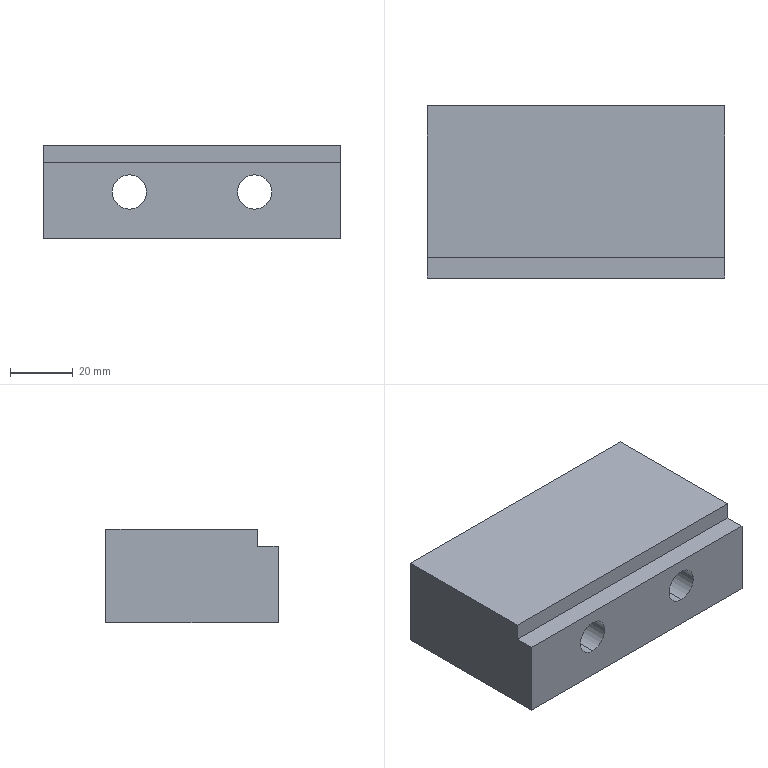Part | SolidWorks | features ICE 3, Extrusion 1 | 1 solid | 18 faces | box 95 x 55 x 30 mm | volume 136523 mm3 | plane 10 | cylinder 8 | commonest cylinder face diameters 11 x4 18 x4
STEP:
#1=CARTESIAN_POINT('',(20.,35.,-9.));
#2=VERTEX_POINT('',#1);
#3=CARTESIAN_POINT('',(20.,35.,9.));
#4=VERTEX_POINT('',#3);
#5=CARTESIAN_POINT('',(20.,35.,0.));
#6=DIRECTION('',(0.,1.,0.));
#7=DIRECTION('',(0.,0.,1.));
#8=AXIS2_PLACEMENT_3D('',#5,#6,#7);
#9=CIRCLE('',#8,9.);
#10=EDGE_CURVE('',#2,#4,#9,.T.);
#11=ORIENTED_EDGE('',*,*,#10,.F.);
#12=CARTESIAN_POINT('',(20.,55.,-9.));
#13=VERTEX_POINT('',#12);
#14=CARTESIAN_POINT('',(20.,35.,-9.));
#15=DIRECTION('',(0.,1.,0.));
#16=VECTOR('',#15,1000.);
#17=LINE('',#14,#16);
#18=EDGE_CURVE('',#2,#13,#17,.T.);
#19=ORIENTED_EDGE('',*,*,#18,.T.);
#20=CARTESIAN_POINT('',(20.,55.,9.));
#21=VERTEX_POINT('',#20);
#22=CARTESIAN_POINT('',(20.,55.,0.));
#23=DIRECTION('',(0.,1.,0.));
#24=DIRECTION('',(0.,0.,1.));
#25=AXIS2_PLACEMENT_3D('',#22,#23,#24);
#26=CIRCLE('',#25,9.);
#27=EDGE_CURVE('',#13,#21,#26,.T.);
#28=ORIENTED_EDGE('',*,*,#27,.T.);
#29=CARTESIAN_POINT('',(20.,35.,9.));
#30=DIRECTION('',(0.,1.,0.));
#31=VECTOR('',#30,1000.);
#32=LINE('',#29,#31);
#33=EDGE_CURVE('',#4,#21,#32,.T.);
#34=ORIENTED_EDGE('',*,*,#33,.F.);
#35=EDGE_LOOP('',(#11,#19,#28,#34));
#36=FACE_OUTER_BOUND('',#35,.T.);
#37=CARTESIAN_POINT('',(20.,35.,0.));
#38=DIRECTION('',(0.,1.,0.));
#39=DIRECTION('',(0.,0.,1.));
#40=AXIS2_PLACEMENT_3D('',#37,#38,#39);
#41=CYLINDRICAL_SURFACE('',#40,9.);
#42=ADVANCED_FACE('',(#36),#41,.F.);
#43=CARTESIAN_POINT('',(-20.,35.,-9.));
#44=VERTEX_POINT('',#43);
#45=CARTESIAN_POINT('',(-20.,35.,9.));
#46=VERTEX_POINT('',#45);
#47=CARTESIAN_POINT('',(-20.,35.,0.));
#48=DIRECTION('',(0.,1.,0.));
#49=DIRECTION('',(0.,0.,1.));
#50=AXIS2_PLACEMENT_3D('',#47,#48,#49);
#51=CIRCLE('',#50,9.);
#52=EDGE_CURVE('',#44,#46,#51,.T.);
#53=ORIENTED_EDGE('',*,*,#52,.F.);
#54=CARTESIAN_POINT('',(-20.,55.,-9.));
#55=VERTEX_POINT('',#54);
#56=CARTESIAN_POINT('',(-20.,35.,-9.));
#57=DIRECTION('',(0.,1.,0.));
#58=VECTOR('',#57,1000.);
#59=LINE('',#56,#58);
#60=EDGE_CURVE('',#44,#55,#59,.T.);
#61=ORIENTED_EDGE('',*,*,#60,.T.);
#62=CARTESIAN_POINT('',(-20.,55.,9.));
#63=VERTEX_POINT('',#62);
#64=CARTESIAN_POINT('',(-20.,55.,0.));
#65=DIRECTION('',(0.,1.,0.));
#66=DIRECTION('',(0.,0.,1.));
#67=AXIS2_PLACEMENT_3D('',#64,#65,#66);
#68=CIRCLE('',#67,9.);
#69=EDGE_CURVE('',#55,#63,#68,.T.);
#70=ORIENTED_EDGE('',*,*,#69,.T.);
#71=CARTESIAN_POINT('',(-20.,35.,9.));
#72=DIRECTION('',(0.,1.,0.));
#73=VECTOR('',#72,1000.);
#74=LINE('',#71,#73);
#75=EDGE_CURVE('',#46,#63,#74,.T.);
#76=ORIENTED_EDGE('',*,*,#75,.F.);
#77=EDGE_LOOP('',(#53,#61,#70,#76));
#78=FACE_OUTER_BOUND('',#77,.T.);
#79=CARTESIAN_POINT('',(-20.,35.,0.));
#80=DIRECTION('',(0.,1.,0.));
#81=DIRECTION('',(0.,0.,1.));
#82=AXIS2_PLACEMENT_3D('',#79,#80,#81);
#83=CYLINDRICAL_SURFACE('',#82,9.);
#84=ADVANCED_FACE('',(#78),#83,.F.);
#85=CARTESIAN_POINT('',(-20.,0.,-5.5));
#86=VERTEX_POINT('',#85);
#87=CARTESIAN_POINT('',(-20.,0.,5.5));
#88=VERTEX_POINT('',#87);
#89=CARTESIAN_POINT('',(-20.,0.,0.));
#90=DIRECTION('',(0.,1.,0.));
#91=DIRECTION('',(0.,0.,1.));
#92=AXIS2_PLACEMENT_3D('',#89,#90,#91);
#93=CIRCLE('',#92,5.5);
#94=EDGE_CURVE('',#86,#88,#93,.T.);
#95=ORIENTED_EDGE('',*,*,#94,.F.);
#96=CARTESIAN_POINT('',(-20.,35.,-5.5));
#97=VERTEX_POINT('',#96);
#98=CARTESIAN_POINT('',(-20.,0.,-5.5));
#99=DIRECTION('',(0.,1.,0.));
#100=VECTOR('',#99,1000.);
#101=LINE('',#98,#100);
#102=EDGE_CURVE('',#86,#97,#101,.T.);
#103=ORIENTED_EDGE('',*,*,#102,.T.);
#104=CARTESIAN_POINT('',(-20.,35.,5.5));
#105=VERTEX_POINT('',#104);
#106=CARTESIAN_POINT('',(-20.,35.,0.));
#107=DIRECTION('',(0.,-1.,0.));
#108=DIRECTION('',(0.,0.,1.));
#109=AXIS2_PLACEMENT_3D('',#106,#107,#108);
#110=CIRCLE('',#109,5.5);
#111=EDGE_CURVE('',#105,#97,#110,.T.);
#112=ORIENTED_EDGE('',*,*,#111,.F.);
#113=CARTESIAN_POINT('',(-20.,0.,5.5));
#114=DIRECTION('',(0.,1.,0.));
#115=VECTOR('',#114,1000.);
#116=LINE('',#113,#115);
#117=EDGE_CURVE('',#88,#105,#116,.T.);
#118=ORIENTED_EDGE('',*,*,#117,.F.);
#119=EDGE_LOOP('',(#95,#103,#112,#118));
#120=FACE_OUTER_BOUND('',#119,.T.);
#121=CARTESIAN_POINT('',(-20.,0.,0.));
#122=DIRECTION('',(0.,1.,0.));
#123=DIRECTION('',(0.,0.,1.));
#124=AXIS2_PLACEMENT_3D('',#121,#122,#123);
#125=CYLINDRICAL_SURFACE('',#124,5.5);
#126=ADVANCED_FACE('',(#120),#125,.F.);
#127=CARTESIAN_POINT('',(20.,0.,-5.5));
#128=VERTEX_POINT('',#127);
#129=CARTESIAN_POINT('',(20.,0.,5.5));
#130=VERTEX_POINT('',#129);
#131=CARTESIAN_POINT('',(20.,0.,0.));
#132=DIRECTION('',(0.,1.,0.));
#133=DIRECTION('',(0.,0.,1.));
#134=AXIS2_PLACEMENT_3D('',#131,#132,#133);
#135=CIRCLE('',#134,5.5);
#136=EDGE_CURVE('',#128,#130,#135,.T.);
#137=ORIENTED_EDGE('',*,*,#136,.F.);
#138=CARTESIAN_POINT('',(20.,35.,-5.5));
#139=VERTEX_POINT('',#138);
#140=CARTESIAN_POINT('',(20.,0.,-5.5));
#141=DIRECTION('',(0.,1.,0.));
#142=VECTOR('',#141,1000.);
#143=LINE('',#140,#142);
#144=EDGE_CURVE('',#128,#139,#143,.T.);
#145=ORIENTED_EDGE('',*,*,#144,.T.);
#146=CARTESIAN_POINT('',(20.,35.,5.5));
#147=VERTEX_POINT('',#146);
#148=CARTESIAN_POINT('',(20.,35.,0.));
#149=DIRECTION('',(0.,-1.,0.));
#150=DIRECTION('',(0.,0.,1.));
#151=AXIS2_PLACEMENT_3D('',#148,#149,#150);
#152=CIRCLE('',#151,5.5);
#153=EDGE_CURVE('',#147,#139,#152,.T.);
#154=ORIENTED_EDGE('',*,*,#153,.F.);
#155=CARTESIAN_POINT('',(20.,0.,5.5));
#156=DIRECTION('',(0.,1.,0.));
#157=VECTOR('',#156,1000.);
#158=LINE('',#155,#157);
#159=EDGE_CURVE('',#130,#147,#158,.T.);
#160=ORIENTED_EDGE('',*,*,#159,.F.);
#161=EDGE_LOOP('',(#137,#145,#154,#160));
#162=FACE_OUTER_BOUND('',#161,.T.);
#163=CARTESIAN_POINT('',(20.,0.,0.));
#164=DIRECTION('',(0.,1.,0.));
#165=DIRECTION('',(0.,0.,1.));
#166=AXIS2_PLACEMENT_3D('',#163,#164,#165);
#167=CYLINDRICAL_SURFACE('',#166,5.5);
#168=ADVANCED_FACE('',(#162),#167,.F.);
#169=ORIENTED_EDGE('',*,*,#144,.F.);
#170=CARTESIAN_POINT('',(20.,0.,0.));
#171=DIRECTION('',(0.,1.,0.));
#172=DIRECTION('',(0.,0.,1.));
#173=AXIS2_PLACEMENT_3D('',#170,#171,#172);
#174=CIRCLE('',#173,5.5);
#175=EDGE_CURVE('',#130,#128,#174,.T.);
#176=ORIENTED_EDGE('',*,*,#175,.F.);
#177=ORIENTED_EDGE('',*,*,#159,.T.);
#178=CARTESIAN_POINT('',(20.,35.,0.));
#179=DIRECTION('',(0.,-1.,0.));
#180=DIRECTION('',(0.,0.,1.));
#181=AXIS2_PLACEMENT_3D('',#178,#179,#180);
#182=CIRCLE('',#181,5.5);
#183=EDGE_CURVE('',#139,#147,#182,.T.);
#184=ORIENTED_EDGE('',*,*,#183,.F.);
#185=EDGE_LOOP('',(#169,#176,#177,#184));
#186=FACE_OUTER_BOUND('',#185,.T.);
#187=CARTESIAN_POINT('',(20.,0.,0.));
#188=DIRECTION('',(0.,1.,0.));
#189=DIRECTION('',(0.,0.,1.));
#190=AXIS2_PLACEMENT_3D('',#187,#188,#189);
#191=CYLINDRICAL_SURFACE('',#190,5.5);
#192=ADVANCED_FACE('',(#186),#191,.F.);
#193=ORIENTED_EDGE('',*,*,#102,.F.);
#194=CARTESIAN_POINT('',(-20.,0.,0.));
#195=DIRECTION('',(0.,1.,0.));
#196=DIRECTION('',(0.,0.,1.));
#197=AXIS2_PLACEMENT_3D('',#194,#195,#196);
#198=CIRCLE('',#197,5.5);
#199=EDGE_CURVE('',#88,#86,#198,.T.);
#200=ORIENTED_EDGE('',*,*,#199,.F.);
#201=ORIENTED_EDGE('',*,*,#117,.T.);
#202=CARTESIAN_POINT('',(-20.,35.,0.));
#203=DIRECTION('',(0.,-1.,0.));
#204=DIRECTION('',(0.,0.,1.));
#205=AXIS2_PLACEMENT_3D('',#202,#203,#204);
#206=CIRCLE('',#205,5.5);
#207=EDGE_CURVE('',#97,#105,#206,.T.);
#208=ORIENTED_EDGE('',*,*,#207,.F.);
#209=EDGE_LOOP('',(#193,#200,#201,#208));
#210=FACE_OUTER_BOUND('',#209,.T.);
#211=CARTESIAN_POINT('',(-20.,0.,0.));
#212=DIRECTION('',(0.,1.,0.));
#213=DIRECTION('',(0.,0.,1.));
#214=AXIS2_PLACEMENT_3D('',#211,#212,#213);
#215=CYLINDRICAL_SURFACE('',#214,5.5);
#216=ADVANCED_FACE('',(#210),#215,.F.);
#217=CARTESIAN_POINT('',(47.5,6.5,15.));
#218=VERTEX_POINT('',#217);
#219=CARTESIAN_POINT('',(47.5,6.5,9.5));
#220=VERTEX_POINT('',#219);
#221=CARTESIAN_POINT('',(47.5,6.5,15.));
#222=DIRECTION('',(0.,0.,-1.));
#223=VECTOR('',#222,1000.);
#224=LINE('',#221,#223);
#225=EDGE_CURVE('',#218,#220,#224,.T.);
#226=ORIENTED_EDGE('',*,*,#225,.T.);
#227=CARTESIAN_POINT('',(47.5,0.,9.5));
#228=VERTEX_POINT('',#227);
#229=CARTESIAN_POINT('',(47.5,55.,9.5));
#230=DIRECTION('',(0.,-1.,0.));
#231=VECTOR('',#230,1000.);
#232=LINE('',#229,#231);
#233=EDGE_CURVE('',#220,#228,#232,.T.);
#234=ORIENTED_EDGE('',*,*,#233,.T.);
#235=CARTESIAN_POINT('',(47.5,0.,-15.));
#236=VERTEX_POINT('',#235);
#237=CARTESIAN_POINT('',(47.5,0.,15.));
#238=DIRECTION('',(0.,0.,-1.));
#239=VECTOR('',#238,1000.);
#240=LINE('',#237,#239);
#241=EDGE_CURVE('',#228,#236,#240,.T.);
#242=ORIENTED_EDGE('',*,*,#241,.T.);
#243=CARTESIAN_POINT('',(47.5,55.,-15.));
#244=VERTEX_POINT('',#243);
#245=CARTESIAN_POINT('',(47.5,55.,-15.));
#246=DIRECTION('',(0.,-1.,0.));
#247=VECTOR('',#246,1000.);
#248=LINE('',#245,#247);
#249=EDGE_CURVE('',#244,#236,#248,.T.);
#250=ORIENTED_EDGE('',*,*,#249,.F.);
#251=CARTESIAN_POINT('',(47.5,55.,15.));
#252=VERTEX_POINT('',#251);
#253=CARTESIAN_POINT('',(47.5,55.,15.));
#254=DIRECTION('',(0.,0.,-1.));
#255=VECTOR('',#254,1000.);
#256=LINE('',#253,#255);
#257=EDGE_CURVE('',#252,#244,#256,.T.);
#258=ORIENTED_EDGE('',*,*,#257,.F.);
#259=CARTESIAN_POINT('',(47.5,55.,15.));
#260=DIRECTION('',(0.,-1.,0.));
#261=VECTOR('',#260,1000.);
#262=LINE('',#259,#261);
#263=EDGE_CURVE('',#252,#218,#262,.T.);
#264=ORIENTED_EDGE('',*,*,#263,.T.);
#265=EDGE_LOOP('',(#226,#234,#242,#250,#258,#264));
#266=FACE_OUTER_BOUND('',#265,.T.);
#267=CARTESIAN_POINT('',(47.5,55.,15.));
#268=DIRECTION('',(-1.,0.,0.));
#269=DIRECTION('',(0.,0.,1.));
#270=AXIS2_PLACEMENT_3D('',#267,#268,#269);
#271=PLANE('',#270);
#272=ADVANCED_FACE('',(#266),#271,.F.);
#273=CARTESIAN_POINT('',(-47.5,0.,-15.));
#274=VERTEX_POINT('',#273);
#275=CARTESIAN_POINT('',(-47.5,0.,-15.));
#276=DIRECTION('',(-1.,0.,0.));
#277=VECTOR('',#276,1000.);
#278=LINE('',#275,#277);
#279=EDGE_CURVE('',#236,#274,#278,.T.);
#280=ORIENTED_EDGE('',*,*,#279,.T.);
#281=CARTESIAN_POINT('',(-47.5,55.,-15.));
#282=VERTEX_POINT('',#281);
#283=CARTESIAN_POINT('',(-47.5,55.,-15.));
#284=DIRECTION('',(0.,-1.,0.));
#285=VECTOR('',#284,1000.);
#286=LINE('',#283,#285);
#287=EDGE_CURVE('',#282,#274,#286,.T.);
#288=ORIENTED_EDGE('',*,*,#287,.F.);
#289=CARTESIAN_POINT('',(-47.5,55.,-15.));
#290=DIRECTION('',(-1.,0.,0.));
#291=VECTOR('',#290,1000.);
#292=LINE('',#289,#291);
#293=EDGE_CURVE('',#244,#282,#292,.T.);
#294=ORIENTED_EDGE('',*,*,#293,.F.);
#295=ORIENTED_EDGE('',*,*,#249,.T.);
#296=EDGE_LOOP('',(#280,#288,#294,#295));
#297=FACE_OUTER_BOUND('',#296,.T.);
#298=CARTESIAN_POINT('',(-47.5,55.,-15.));
#299=DIRECTION('',(0.,0.,1.));
#300=DIRECTION('',(1.,0.,0.));
#301=AXIS2_PLACEMENT_3D('',#298,#299,#300);
#302=PLANE('',#301);
#303=ADVANCED_FACE('',(#297),#302,.F.);
#304=CARTESIAN_POINT('',(-47.5,0.,9.5));
#305=VERTEX_POINT('',#304);
#306=CARTESIAN_POINT('',(-47.5,0.,15.));
#307=DIRECTION('',(0.,0.,1.));
#308=VECTOR('',#307,1000.);
#309=LINE('',#306,#308);
#310=EDGE_CURVE('',#274,#305,#309,.T.);
#311=ORIENTED_EDGE('',*,*,#310,.T.);
#312=CARTESIAN_POINT('',(-47.5,6.5,9.5));
#313=VERTEX_POINT('',#312);
#314=CARTESIAN_POINT('',(-47.5,0.,9.5));
#315=DIRECTION('',(0.,-1.,0.));
#316=VECTOR('',#315,1000.);
#317=LINE('',#314,#316);
#318=EDGE_CURVE('',#313,#305,#317,.T.);
#319=ORIENTED_EDGE('',*,*,#318,.F.);
#320=CARTESIAN_POINT('',(-47.5,6.5,15.));
#321=VERTEX_POINT('',#320);
#322=CARTESIAN_POINT('',(-47.5,6.5,15.));
#323=DIRECTION('',(0.,0.,-1.));
#324=VECTOR('',#323,1000.);
#325=LINE('',#322,#324);
#326=EDGE_CURVE('',#321,#313,#325,.T.);
#327=ORIENTED_EDGE('',*,*,#326,.F.);
#328=CARTESIAN_POINT('',(-47.5,55.,15.));
#329=VERTEX_POINT('',#328);
#330=CARTESIAN_POINT('',(-47.5,55.,15.));
#331=DIRECTION('',(0.,-1.,0.));
#332=VECTOR('',#331,1000.);
#333=LINE('',#330,#332);
#334=EDGE_CURVE('',#329,#321,#333,.T.);
#335=ORIENTED_EDGE('',*,*,#334,.F.);
#336=CARTESIAN_POINT('',(-47.5,55.,15.));
#337=DIRECTION('',(0.,0.,1.));
#338=VECTOR('',#337,1000.);
#339=LINE('',#336,#338);
#340=EDGE_CURVE('',#282,#329,#339,.T.);
#341=ORIENTED_EDGE('',*,*,#340,.F.);
#342=ORIENTED_EDGE('',*,*,#287,.T.);
#343=EDGE_LOOP('',(#311,#319,#327,#335,#341,#342));
#344=FACE_OUTER_BOUND('',#343,.T.);
#345=CARTESIAN_POINT('',(-47.5,55.,15.));
#346=DIRECTION('',(1.,0.,0.));
#347=DIRECTION('',(0.,0.,-1.));
#348=AXIS2_PLACEMENT_3D('',#345,#346,#347);
#349=PLANE('',#348);
#350=ADVANCED_FACE('',(#344),#349,.F.);
#351=ORIENTED_EDGE('',*,*,#334,.T.);
#352=CARTESIAN_POINT('',(124.5,6.5,15.));
#353=DIRECTION('',(-1.,0.,0.));
#354=VECTOR('',#353,1000.);
#355=LINE('',#352,#354);
#356=EDGE_CURVE('',#218,#321,#355,.T.);
#357=ORIENTED_EDGE('',*,*,#356,.F.);
#358=ORIENTED_EDGE('',*,*,#263,.F.);
#359=CARTESIAN_POINT('',(-47.5,55.,15.));
#360=DIRECTION('',(1.,0.,0.));
#361=VECTOR('',#360,1000.);
#362=LINE('',#359,#361);
#363=EDGE_CURVE('',#329,#252,#362,.T.);
#364=ORIENTED_EDGE('',*,*,#363,.F.);
#365=EDGE_LOOP('',(#351,#357,#358,#364));
#366=FACE_OUTER_BOUND('',#365,.T.);
#367=CARTESIAN_POINT('',(-47.5,55.,15.));
#368=DIRECTION('',(0.,0.,-1.));
#369=DIRECTION('',(-1.,0.,0.));
#370=AXIS2_PLACEMENT_3D('',#367,#368,#369);
#371=PLANE('',#370);
#372=ADVANCED_FACE('',(#366),#371,.F.);
#373=CARTESIAN_POINT('',(-20.,55.,0.));
#374=DIRECTION('',(0.,1.,0.));
#375=DIRECTION('',(0.,0.,1.));
#376=AXIS2_PLACEMENT_3D('',#373,#374,#375);
#377=CIRCLE('',#376,9.);
#378=EDGE_CURVE('',#63,#55,#377,.T.);
#379=ORIENTED_EDGE('',*,*,#378,.F.);
#380=ORIENTED_EDGE('',*,*,#69,.F.);
#381=EDGE_LOOP('',(#379,#380));
#382=FACE_BOUND('',#381,.T.);
#383=CARTESIAN_POINT('',(20.,55.,0.));
#384=DIRECTION('',(0.,1.,0.));
#385=DIRECTION('',(0.,0.,1.));
#386=AXIS2_PLACEMENT_3D('',#383,#384,#385);
#387=CIRCLE('',#386,9.);
#388=EDGE_CURVE('',#21,#13,#387,.T.);
#389=ORIENTED_EDGE('',*,*,#388,.F.);
#390=ORIENTED_EDGE('',*,*,#27,.F.);
#391=EDGE_LOOP('',(#389,#390));
#392=FACE_BOUND('',#391,.T.);
#393=ORIENTED_EDGE('',*,*,#257,.T.);
#394=ORIENTED_EDGE('',*,*,#293,.T.);
#395=ORIENTED_EDGE('',*,*,#340,.T.);
#396=ORIENTED_EDGE('',*,*,#363,.T.);
#397=EDGE_LOOP('',(#393,#394,#395,#396));
#398=FACE_OUTER_BOUND('',#397,.T.);
#399=CARTESIAN_POINT('',(0.,55.,0.));
#400=DIRECTION('',(0.,-1.,0.));
#401=DIRECTION('',(0.,0.,-1.));
#402=AXIS2_PLACEMENT_3D('',#399,#400,#401);
#403=PLANE('',#402);
#404=ADVANCED_FACE('',(#382,#392,#398),#403,.F.);
#405=CARTESIAN_POINT('',(0.,0.,9.5));
#406=DIRECTION('',(1.,0.,0.));
#407=VECTOR('',#406,1000.);
#408=LINE('',#405,#407);
#409=EDGE_CURVE('',#305,#228,#408,.T.);
#410=ORIENTED_EDGE('',*,*,#409,.F.);
#411=ORIENTED_EDGE('',*,*,#310,.F.);
#412=ORIENTED_EDGE('',*,*,#279,.F.);
#413=ORIENTED_EDGE('',*,*,#241,.F.);
#414=EDGE_LOOP('',(#410,#411,#412,#413));
#415=FACE_OUTER_BOUND('',#414,.T.);
#416=ORIENTED_EDGE('',*,*,#199,.T.);
#417=ORIENTED_EDGE('',*,*,#94,.T.);
#418=EDGE_LOOP('',(#416,#417));
#419=FACE_BOUND('',#418,.T.);
#420=ORIENTED_EDGE('',*,*,#175,.T.);
#421=ORIENTED_EDGE('',*,*,#136,.T.);
#422=EDGE_LOOP('',(#420,#421));
#423=FACE_BOUND('',#422,.T.);
#424=CARTESIAN_POINT('',(0.,0.,0.));
#425=DIRECTION('',(0.,-1.,0.));
#426=DIRECTION('',(0.,0.,-1.));
#427=AXIS2_PLACEMENT_3D('',#424,#425,#426);
#428=PLANE('',#427);
#429=ADVANCED_FACE('',(#415,#419,#423),#428,.T.);
#430=CARTESIAN_POINT('',(-20.,35.,0.));
#431=DIRECTION('',(0.,1.,0.));
#432=DIRECTION('',(0.,0.,1.));
#433=AXIS2_PLACEMENT_3D('',#430,#431,#432);
#434=CIRCLE('',#433,9.);
#435=EDGE_CURVE('',#46,#44,#434,.T.);
#436=ORIENTED_EDGE('',*,*,#435,.T.);
#437=ORIENTED_EDGE('',*,*,#52,.T.);
#438=EDGE_LOOP('',(#436,#437));
#439=FACE_OUTER_BOUND('',#438,.T.);
#440=ORIENTED_EDGE('',*,*,#111,.T.);
#441=ORIENTED_EDGE('',*,*,#207,.T.);
#442=EDGE_LOOP('',(#440,#441));
#443=FACE_BOUND('',#442,.T.);
#444=CARTESIAN_POINT('',(-20.,35.,0.));
#445=DIRECTION('',(0.,1.,0.));
#446=DIRECTION('',(0.,0.,1.));
#447=AXIS2_PLACEMENT_3D('',#444,#445,#446);
#448=PLANE('',#447);
#449=ADVANCED_FACE('',(#439,#443),#448,.T.);
#450=ORIENTED_EDGE('',*,*,#60,.F.);
#451=ORIENTED_EDGE('',*,*,#435,.F.);
#452=ORIENTED_EDGE('',*,*,#75,.T.);
#453=ORIENTED_EDGE('',*,*,#378,.T.);
#454=EDGE_LOOP('',(#450,#451,#452,#453));
#455=FACE_OUTER_BOUND('',#454,.T.);
#456=CARTESIAN_POINT('',(-20.,35.,0.));
#457=DIRECTION('',(0.,1.,0.));
#458=DIRECTION('',(0.,0.,1.));
#459=AXIS2_PLACEMENT_3D('',#456,#457,#458);
#460=CYLINDRICAL_SURFACE('',#459,9.);
#461=ADVANCED_FACE('',(#455),#460,.F.);
#462=CARTESIAN_POINT('',(20.,35.,0.));
#463=DIRECTION('',(0.,1.,0.));
#464=DIRECTION('',(0.,0.,1.));
#465=AXIS2_PLACEMENT_3D('',#462,#463,#464);
#466=CIRCLE('',#465,9.);
#467=EDGE_CURVE('',#4,#2,#466,.T.);
#468=ORIENTED_EDGE('',*,*,#467,.T.);
#469=ORIENTED_EDGE('',*,*,#10,.T.);
#470=EDGE_LOOP('',(#468,#469));
#471=FACE_OUTER_BOUND('',#470,.T.);
#472=ORIENTED_EDGE('',*,*,#153,.T.);
#473=ORIENTED_EDGE('',*,*,#183,.T.);
#474=EDGE_LOOP('',(#472,#473));
#475=FACE_BOUND('',#474,.T.);
#476=CARTESIAN_POINT('',(20.,35.,0.));
#477=DIRECTION('',(0.,1.,0.));
#478=DIRECTION('',(0.,0.,1.));
#479=AXIS2_PLACEMENT_3D('',#476,#477,#478);
#480=PLANE('',#479);
#481=ADVANCED_FACE('',(#471,#475),#480,.T.);
#482=ORIENTED_EDGE('',*,*,#18,.F.);
#483=ORIENTED_EDGE('',*,*,#467,.F.);
#484=ORIENTED_EDGE('',*,*,#33,.T.);
#485=ORIENTED_EDGE('',*,*,#388,.T.);
#486=EDGE_LOOP('',(#482,#483,#484,#485));
#487=FACE_OUTER_BOUND('',#486,.T.);
#488=CARTESIAN_POINT('',(20.,35.,0.));
#489=DIRECTION('',(0.,1.,0.));
#490=DIRECTION('',(0.,0.,1.));
#491=AXIS2_PLACEMENT_3D('',#488,#489,#490);
#492=CYLINDRICAL_SURFACE('',#491,9.);
#493=ADVANCED_FACE('',(#487),#492,.F.);
#494=ORIENTED_EDGE('',*,*,#356,.T.);
#495=ORIENTED_EDGE('',*,*,#326,.T.);
#496=CARTESIAN_POINT('',(124.5,6.5,9.5));
#497=DIRECTION('',(-1.,0.,0.));
#498=VECTOR('',#497,1000.);
#499=LINE('',#496,#498);
#500=EDGE_CURVE('',#220,#313,#499,.T.);
#501=ORIENTED_EDGE('',*,*,#500,.F.);
#502=ORIENTED_EDGE('',*,*,#225,.F.);
#503=EDGE_LOOP('',(#494,#495,#501,#502));
#504=FACE_OUTER_BOUND('',#503,.T.);
#505=CARTESIAN_POINT('',(124.5,6.5,15.));
#506=DIRECTION('',(0.,1.,0.));
#507=DIRECTION('',(0.,0.,1.));
#508=AXIS2_PLACEMENT_3D('',#505,#506,#507);
#509=PLANE('',#508);
#510=ADVANCED_FACE('',(#504),#509,.F.);
#511=ORIENTED_EDGE('',*,*,#500,.T.);
#512=ORIENTED_EDGE('',*,*,#318,.T.);
#513=ORIENTED_EDGE('',*,*,#409,.T.);
#514=ORIENTED_EDGE('',*,*,#233,.F.);
#515=EDGE_LOOP('',(#511,#512,#513,#514));
#516=FACE_OUTER_BOUND('',#515,.T.);
#517=CARTESIAN_POINT('',(124.5,0.,9.5));
#518=DIRECTION('',(0.,0.,-1.));
#519=DIRECTION('',(-1.,0.,0.));
#520=AXIS2_PLACEMENT_3D('',#517,#518,#519);
#521=PLANE('',#520);
#522=ADVANCED_FACE('',(#516),#521,.F.);
#523=CLOSED_SHELL('',(#42,#84,#126,#168,#192,#216,#272,#303,#350,#372,#404,#429,#449,#461,#481,#493,#510,#522));
#524=MANIFOLD_SOLID_BREP('',#523);
#525=CARTESIAN_POINT('',(0.,0.,0.));
#526=DIRECTION('',(0.,0.,1.));
#527=DIRECTION('',(1.,0.,0.));
#528=AXIS2_PLACEMENT_3D('',#525,#526,#527);
#529=(LENGTH_UNIT()NAMED_UNIT(*)SI_UNIT(.MILLI.,.METRE.));
#530=UNCERTAINTY_MEASURE_WITH_UNIT(LENGTH_MEASURE(0.00001),#529,'','');
#531=(NAMED_UNIT(*)PLANE_ANGLE_UNIT()SI_UNIT($,.RADIAN.));
#532=(NAMED_UNIT(*)SI_UNIT($,.STERADIAN.)SOLID_ANGLE_UNIT());
#533=(GEOMETRIC_REPRESENTATION_CONTEXT(3)GLOBAL_UNCERTAINTY_ASSIGNED_CONTEXT((#530))GLOBAL_UNIT_ASSIGNED_CONTEXT((#529,#531,#532))REPRESENTATION_CONTEXT('',''));
#534=ADVANCED_BREP_SHAPE_REPRESENTATION('',(#524,#528),#533);